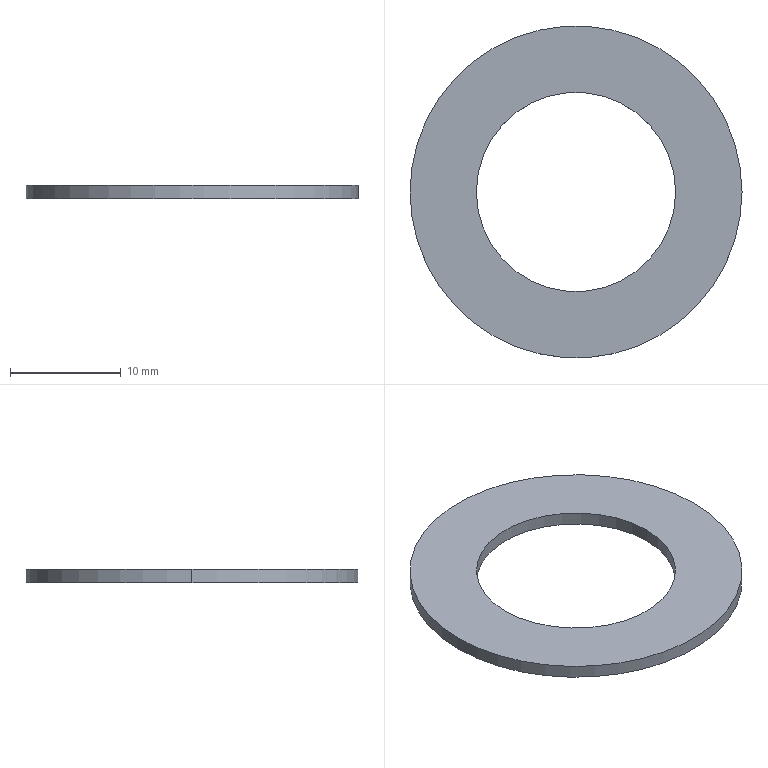Part | SolidWorks | features Extrusion 1 | 1 solid | 6 faces | box 30 x 30 x 1.2 mm | volume 542.867 mm3 | cylinder 4 | plane 2 | commonest cylinder face diameters 18 x2 30 x2
STEP:
#1=CARTESIAN_POINT('',(-12.15,-4.234,1.2));
#2=VERTEX_POINT('',#1);
#3=CARTESIAN_POINT('',(5.85,-4.234,1.2));
#4=VERTEX_POINT('',#3);
#5=CARTESIAN_POINT('',(-3.15,-4.234,1.2));
#6=DIRECTION('',(0.,0.,1.));
#7=DIRECTION('',(1.,0.,0.));
#8=AXIS2_PLACEMENT_3D('',#5,#6,#7);
#9=CIRCLE('',#8,9.);
#10=EDGE_CURVE('',#2,#4,#9,.T.);
#11=ORIENTED_EDGE('',*,*,#10,.T.);
#12=CARTESIAN_POINT('',(5.85,-4.234,0.));
#13=VERTEX_POINT('',#12);
#14=CARTESIAN_POINT('',(5.85,-4.234,1.2));
#15=DIRECTION('',(0.,0.,-1.));
#16=VECTOR('',#15,1000.);
#17=LINE('',#14,#16);
#18=EDGE_CURVE('',#4,#13,#17,.T.);
#19=ORIENTED_EDGE('',*,*,#18,.T.);
#20=CARTESIAN_POINT('',(-12.15,-4.234,0.));
#21=VERTEX_POINT('',#20);
#22=CARTESIAN_POINT('',(-3.15,-4.234,0.));
#23=DIRECTION('',(0.,0.,1.));
#24=DIRECTION('',(1.,0.,0.));
#25=AXIS2_PLACEMENT_3D('',#22,#23,#24);
#26=CIRCLE('',#25,9.);
#27=EDGE_CURVE('',#21,#13,#26,.T.);
#28=ORIENTED_EDGE('',*,*,#27,.F.);
#29=CARTESIAN_POINT('',(-12.15,-4.234,1.2));
#30=DIRECTION('',(0.,0.,-1.));
#31=VECTOR('',#30,1000.);
#32=LINE('',#29,#31);
#33=EDGE_CURVE('',#2,#21,#32,.T.);
#34=ORIENTED_EDGE('',*,*,#33,.F.);
#35=EDGE_LOOP('',(#11,#19,#28,#34));
#36=FACE_OUTER_BOUND('',#35,.T.);
#37=CARTESIAN_POINT('',(-3.15,-4.234,1.2));
#38=DIRECTION('',(0.,0.,-1.));
#39=DIRECTION('',(-1.,0.,0.));
#40=AXIS2_PLACEMENT_3D('',#37,#38,#39);
#41=CYLINDRICAL_SURFACE('',#40,9.);
#42=ADVANCED_FACE('',(#36),#41,.F.);
#43=CARTESIAN_POINT('',(11.85,-4.234,1.2));
#44=VERTEX_POINT('',#43);
#45=CARTESIAN_POINT('',(-18.15,-4.234,1.2));
#46=VERTEX_POINT('',#45);
#47=CARTESIAN_POINT('',(-3.15,-4.234,1.2));
#48=DIRECTION('',(0.,0.,1.));
#49=DIRECTION('',(1.,0.,0.));
#50=AXIS2_PLACEMENT_3D('',#47,#48,#49);
#51=CIRCLE('',#50,15.);
#52=EDGE_CURVE('',#44,#46,#51,.T.);
#53=ORIENTED_EDGE('',*,*,#52,.F.);
#54=CARTESIAN_POINT('',(11.85,-4.234,0.));
#55=VERTEX_POINT('',#54);
#56=CARTESIAN_POINT('',(11.85,-4.234,1.2));
#57=DIRECTION('',(0.,0.,-1.));
#58=VECTOR('',#57,1000.);
#59=LINE('',#56,#58);
#60=EDGE_CURVE('',#44,#55,#59,.T.);
#61=ORIENTED_EDGE('',*,*,#60,.T.);
#62=CARTESIAN_POINT('',(-18.15,-4.234,0.));
#63=VERTEX_POINT('',#62);
#64=CARTESIAN_POINT('',(-3.15,-4.234,0.));
#65=DIRECTION('',(0.,0.,1.));
#66=DIRECTION('',(1.,0.,0.));
#67=AXIS2_PLACEMENT_3D('',#64,#65,#66);
#68=CIRCLE('',#67,15.);
#69=EDGE_CURVE('',#55,#63,#68,.T.);
#70=ORIENTED_EDGE('',*,*,#69,.T.);
#71=CARTESIAN_POINT('',(-18.15,-4.234,1.2));
#72=DIRECTION('',(0.,0.,-1.));
#73=VECTOR('',#72,1000.);
#74=LINE('',#71,#73);
#75=EDGE_CURVE('',#46,#63,#74,.T.);
#76=ORIENTED_EDGE('',*,*,#75,.F.);
#77=EDGE_LOOP('',(#53,#61,#70,#76));
#78=FACE_OUTER_BOUND('',#77,.T.);
#79=CARTESIAN_POINT('',(-3.15,-4.234,1.2));
#80=DIRECTION('',(0.,0.,-1.));
#81=DIRECTION('',(-1.,0.,0.));
#82=AXIS2_PLACEMENT_3D('',#79,#80,#81);
#83=CYLINDRICAL_SURFACE('',#82,15.);
#84=ADVANCED_FACE('',(#78),#83,.T.);
#85=CARTESIAN_POINT('',(-3.15,-4.234,1.2));
#86=DIRECTION('',(0.,0.,1.));
#87=DIRECTION('',(1.,0.,0.));
#88=AXIS2_PLACEMENT_3D('',#85,#86,#87);
#89=CIRCLE('',#88,15.);
#90=EDGE_CURVE('',#46,#44,#89,.T.);
#91=ORIENTED_EDGE('',*,*,#90,.T.);
#92=ORIENTED_EDGE('',*,*,#52,.T.);
#93=EDGE_LOOP('',(#91,#92));
#94=FACE_OUTER_BOUND('',#93,.T.);
#95=ORIENTED_EDGE('',*,*,#10,.F.);
#96=CARTESIAN_POINT('',(-3.15,-4.234,1.2));
#97=DIRECTION('',(0.,0.,1.));
#98=DIRECTION('',(1.,0.,0.));
#99=AXIS2_PLACEMENT_3D('',#96,#97,#98);
#100=CIRCLE('',#99,9.);
#101=EDGE_CURVE('',#4,#2,#100,.T.);
#102=ORIENTED_EDGE('',*,*,#101,.F.);
#103=EDGE_LOOP('',(#95,#102));
#104=FACE_BOUND('',#103,.T.);
#105=CARTESIAN_POINT('',(-3.15,-4.234,1.2));
#106=DIRECTION('',(0.,0.,1.));
#107=DIRECTION('',(1.,0.,0.));
#108=AXIS2_PLACEMENT_3D('',#105,#106,#107);
#109=PLANE('',#108);
#110=ADVANCED_FACE('',(#94,#104),#109,.T.);
#111=CARTESIAN_POINT('',(-3.15,-4.234,0.));
#112=DIRECTION('',(0.,0.,1.));
#113=DIRECTION('',(1.,0.,0.));
#114=AXIS2_PLACEMENT_3D('',#111,#112,#113);
#115=CIRCLE('',#114,15.);
#116=EDGE_CURVE('',#63,#55,#115,.T.);
#117=ORIENTED_EDGE('',*,*,#116,.F.);
#118=ORIENTED_EDGE('',*,*,#69,.F.);
#119=EDGE_LOOP('',(#117,#118));
#120=FACE_OUTER_BOUND('',#119,.T.);
#121=ORIENTED_EDGE('',*,*,#27,.T.);
#122=CARTESIAN_POINT('',(-3.15,-4.234,0.));
#123=DIRECTION('',(0.,0.,1.));
#124=DIRECTION('',(1.,0.,0.));
#125=AXIS2_PLACEMENT_3D('',#122,#123,#124);
#126=CIRCLE('',#125,9.);
#127=EDGE_CURVE('',#13,#21,#126,.T.);
#128=ORIENTED_EDGE('',*,*,#127,.T.);
#129=EDGE_LOOP('',(#121,#128));
#130=FACE_BOUND('',#129,.T.);
#131=CARTESIAN_POINT('',(-3.15,-4.234,0.));
#132=DIRECTION('',(0.,0.,1.));
#133=DIRECTION('',(1.,0.,0.));
#134=AXIS2_PLACEMENT_3D('',#131,#132,#133);
#135=PLANE('',#134);
#136=ADVANCED_FACE('',(#120,#130),#135,.F.);
#137=ORIENTED_EDGE('',*,*,#60,.F.);
#138=ORIENTED_EDGE('',*,*,#90,.F.);
#139=ORIENTED_EDGE('',*,*,#75,.T.);
#140=ORIENTED_EDGE('',*,*,#116,.T.);
#141=EDGE_LOOP('',(#137,#138,#139,#140));
#142=FACE_OUTER_BOUND('',#141,.T.);
#143=CARTESIAN_POINT('',(-3.15,-4.234,1.2));
#144=DIRECTION('',(0.,0.,-1.));
#145=DIRECTION('',(-1.,0.,0.));
#146=AXIS2_PLACEMENT_3D('',#143,#144,#145);
#147=CYLINDRICAL_SURFACE('',#146,15.);
#148=ADVANCED_FACE('',(#142),#147,.T.);
#149=ORIENTED_EDGE('',*,*,#18,.F.);
#150=ORIENTED_EDGE('',*,*,#101,.T.);
#151=ORIENTED_EDGE('',*,*,#33,.T.);
#152=ORIENTED_EDGE('',*,*,#127,.F.);
#153=EDGE_LOOP('',(#149,#150,#151,#152));
#154=FACE_OUTER_BOUND('',#153,.T.);
#155=CARTESIAN_POINT('',(-3.15,-4.234,1.2));
#156=DIRECTION('',(0.,0.,-1.));
#157=DIRECTION('',(-1.,0.,0.));
#158=AXIS2_PLACEMENT_3D('',#155,#156,#157);
#159=CYLINDRICAL_SURFACE('',#158,9.);
#160=ADVANCED_FACE('',(#154),#159,.F.);
#161=CLOSED_SHELL('',(#42,#84,#110,#136,#148,#160));
#162=MANIFOLD_SOLID_BREP('',#161);
#163=CARTESIAN_POINT('',(0.,0.,0.));
#164=DIRECTION('',(0.,0.,1.));
#165=DIRECTION('',(1.,0.,0.));
#166=AXIS2_PLACEMENT_3D('',#163,#164,#165);
#167=(LENGTH_UNIT()NAMED_UNIT(*)SI_UNIT(.MILLI.,.METRE.));
#168=UNCERTAINTY_MEASURE_WITH_UNIT(LENGTH_MEASURE(0.00001),#167,'','');
#169=(NAMED_UNIT(*)PLANE_ANGLE_UNIT()SI_UNIT($,.RADIAN.));
#170=(NAMED_UNIT(*)SI_UNIT($,.STERADIAN.)SOLID_ANGLE_UNIT());
#171=(GEOMETRIC_REPRESENTATION_CONTEXT(3)GLOBAL_UNCERTAINTY_ASSIGNED_CONTEXT((#168))GLOBAL_UNIT_ASSIGNED_CONTEXT((#167,#169,#170))REPRESENTATION_CONTEXT('',''));
#172=ADVANCED_BREP_SHAPE_REPRESENTATION('',(#162,#166),#171);